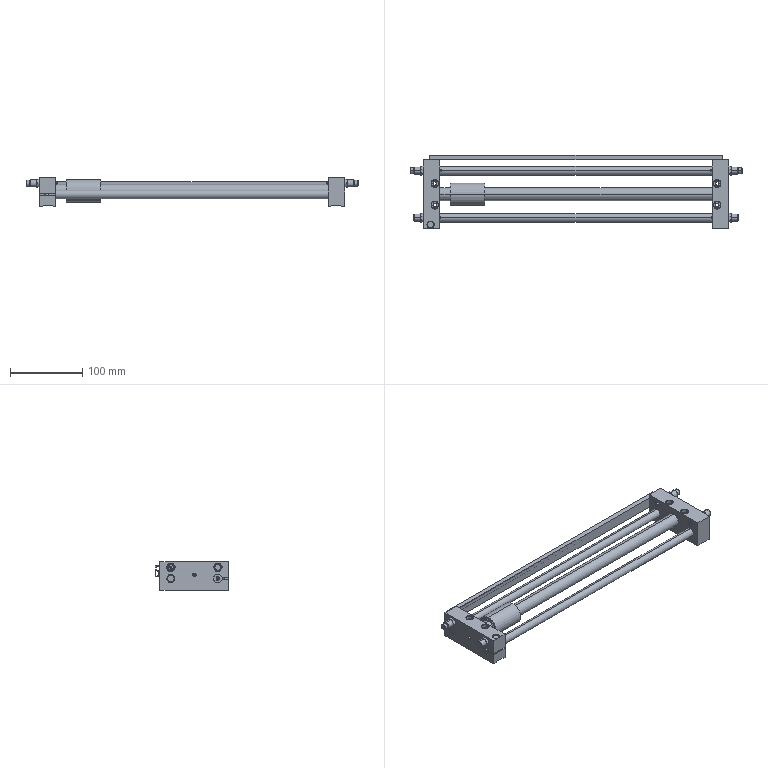Part | STEP file | 1 solid | 352 faces | box 459 x 101.4 x 39 mm | volume 391134 mm3 | cylinder 116 | plane 116 | cone 108 | torus 12 | commonest cylinder face diameters 12 x30 10 x12 3 x8 4.917 x8 5.5 x8 8.376 x8